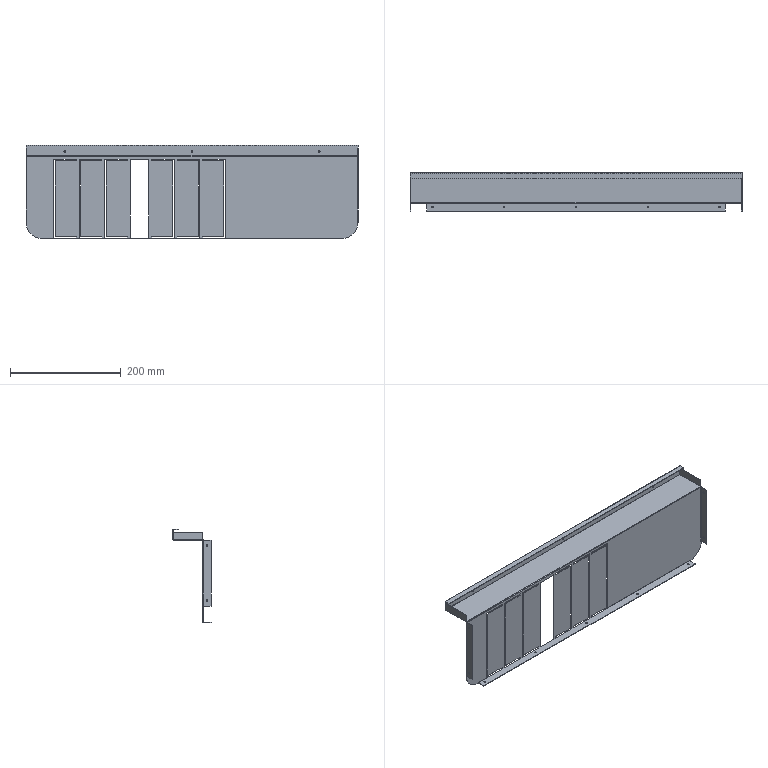Part | STEP file | HESS-408-70-15W-N-6-inner liner turbine outlet baffle | 1 solid | 154 faces | box 600 x 69 x 169 mm | volume 141384 mm3 | plane 98 | cylinder 56 | commonest cylinder face diameters 3.2 x24 0.2 x15 2.2 x15 60 x2